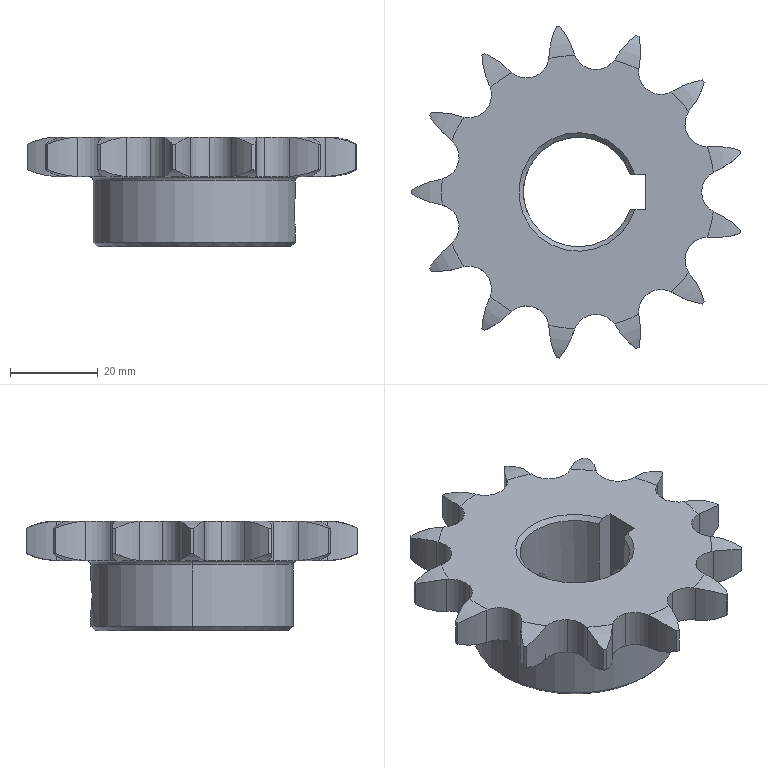Part | STEP file | 5-fen-13-tooth_GearTrax | 1 solid | 111 faces | box 75.004 x 75.553 x 24.975 mm | volume 40881 mm3 | cylinder 72 | torus 28 | plane 6 | cone 5 | commonest cylinder face diameters 10.262 x26 36.576 x26 76.019 x13 6.8 x4 46 x2 25 x1